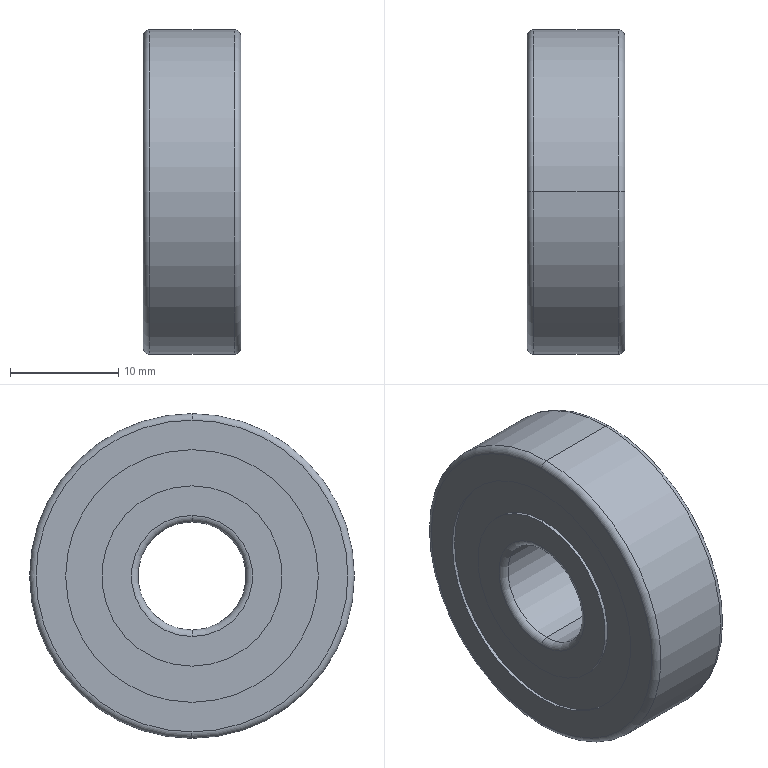Part | SolidWorks | features Revolution 3, CirPattern 1, RefAxis 1 | 16 solids | 86 faces | box 9 x 30 x 30 mm | volume 4367 mm3 | sphere 26 | cylinder 24 | torus 14 | cone 12 | plane 10 | commonest cylinder face diameters 16.667 x6 23.333 x6 15.467 x4 24.533 x4 10 x2 30 x2